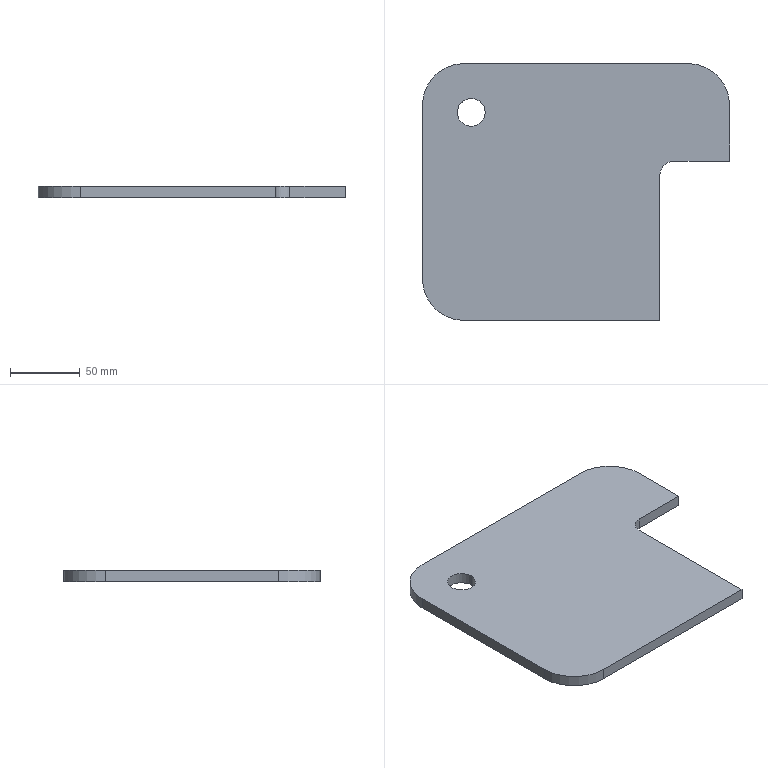Part | SolidWorks | features Extrusion 1 | 1 solid | 14 faces | box 220 x 184 x 8 mm | volume 271263 mm3 | plane 8 | cylinder 6 | commonest cylinder face diameters 20 x3 60 x3
STEP:
#1=CARTESIAN_POINT('',(25.,149.,8.));
#2=VERTEX_POINT('',#1);
#3=CARTESIAN_POINT('',(45.,149.,8.));
#4=VERTEX_POINT('',#3);
#5=CARTESIAN_POINT('',(35.,149.,8.));
#6=DIRECTION('',(0.,0.,1.));
#7=DIRECTION('',(1.,0.,0.));
#8=AXIS2_PLACEMENT_3D('',#5,#6,#7);
#9=CIRCLE('',#8,10.);
#10=EDGE_CURVE('',#2,#4,#9,.T.);
#11=ORIENTED_EDGE('',*,*,#10,.T.);
#12=CARTESIAN_POINT('',(45.,149.,0.));
#13=VERTEX_POINT('',#12);
#14=CARTESIAN_POINT('',(45.,149.,8.));
#15=DIRECTION('',(0.,0.,-1.));
#16=VECTOR('',#15,1000.);
#17=LINE('',#14,#16);
#18=EDGE_CURVE('',#4,#13,#17,.T.);
#19=ORIENTED_EDGE('',*,*,#18,.T.);
#20=CARTESIAN_POINT('',(25.,149.,0.));
#21=VERTEX_POINT('',#20);
#22=CARTESIAN_POINT('',(35.,149.,0.));
#23=DIRECTION('',(0.,0.,1.));
#24=DIRECTION('',(1.,0.,0.));
#25=AXIS2_PLACEMENT_3D('',#22,#23,#24);
#26=CIRCLE('',#25,10.);
#27=EDGE_CURVE('',#21,#13,#26,.T.);
#28=ORIENTED_EDGE('',*,*,#27,.F.);
#29=CARTESIAN_POINT('',(25.,149.,8.));
#30=DIRECTION('',(0.,0.,-1.));
#31=VECTOR('',#30,1000.);
#32=LINE('',#29,#31);
#33=EDGE_CURVE('',#2,#21,#32,.T.);
#34=ORIENTED_EDGE('',*,*,#33,.F.);
#35=EDGE_LOOP('',(#11,#19,#28,#34));
#36=FACE_OUTER_BOUND('',#35,.T.);
#37=CARTESIAN_POINT('',(35.,149.,8.));
#38=DIRECTION('',(0.,0.,-1.));
#39=DIRECTION('',(-1.,0.,0.));
#40=AXIS2_PLACEMENT_3D('',#37,#38,#39);
#41=CYLINDRICAL_SURFACE('',#40,10.);
#42=ADVANCED_FACE('',(#36),#41,.F.);
#43=CARTESIAN_POINT('',(220.,154.,8.));
#44=VERTEX_POINT('',#43);
#45=CARTESIAN_POINT('',(190.,184.,8.));
#46=VERTEX_POINT('',#45);
#47=CARTESIAN_POINT('',(190.,154.,8.));
#48=DIRECTION('',(0.,0.,1.));
#49=DIRECTION('',(-1.,0.,0.));
#50=AXIS2_PLACEMENT_3D('',#47,#48,#49);
#51=CIRCLE('',#50,30.);
#52=EDGE_CURVE('',#44,#46,#51,.T.);
#53=ORIENTED_EDGE('',*,*,#52,.T.);
#54=CARTESIAN_POINT('',(30.,184.,8.));
#55=VERTEX_POINT('',#54);
#56=CARTESIAN_POINT('',(30.,184.,8.));
#57=DIRECTION('',(-1.,0.,0.));
#58=VECTOR('',#57,1000.);
#59=LINE('',#56,#58);
#60=EDGE_CURVE('',#46,#55,#59,.T.);
#61=ORIENTED_EDGE('',*,*,#60,.T.);
#62=CARTESIAN_POINT('',(0.,154.,8.));
#63=VERTEX_POINT('',#62);
#64=CARTESIAN_POINT('',(30.,154.,8.));
#65=DIRECTION('',(0.,0.,1.));
#66=DIRECTION('',(-1.,0.,0.));
#67=AXIS2_PLACEMENT_3D('',#64,#65,#66);
#68=CIRCLE('',#67,30.);
#69=EDGE_CURVE('',#55,#63,#68,.T.);
#70=ORIENTED_EDGE('',*,*,#69,.T.);
#71=CARTESIAN_POINT('',(0.,30.,8.));
#72=VERTEX_POINT('',#71);
#73=CARTESIAN_POINT('',(0.,30.,8.));
#74=DIRECTION('',(0.,-1.,0.));
#75=VECTOR('',#74,1000.);
#76=LINE('',#73,#75);
#77=EDGE_CURVE('',#63,#72,#76,.T.);
#78=ORIENTED_EDGE('',*,*,#77,.T.);
#79=CARTESIAN_POINT('',(30.,0.,8.));
#80=VERTEX_POINT('',#79);
#81=CARTESIAN_POINT('',(30.,30.,8.));
#82=DIRECTION('',(0.,0.,1.));
#83=DIRECTION('',(1.,0.,0.));
#84=AXIS2_PLACEMENT_3D('',#81,#82,#83);
#85=CIRCLE('',#84,30.);
#86=EDGE_CURVE('',#72,#80,#85,.T.);
#87=ORIENTED_EDGE('',*,*,#86,.T.);
#88=CARTESIAN_POINT('',(170.,0.,8.));
#89=VERTEX_POINT('',#88);
#90=CARTESIAN_POINT('',(170.,0.,8.));
#91=DIRECTION('',(1.,0.,0.));
#92=VECTOR('',#91,1000.);
#93=LINE('',#90,#92);
#94=EDGE_CURVE('',#80,#89,#93,.T.);
#95=ORIENTED_EDGE('',*,*,#94,.T.);
#96=CARTESIAN_POINT('',(170.,104.,8.));
#97=VERTEX_POINT('',#96);
#98=CARTESIAN_POINT('',(170.,104.,8.));
#99=DIRECTION('',(0.,1.,0.));
#100=VECTOR('',#99,1000.);
#101=LINE('',#98,#100);
#102=EDGE_CURVE('',#89,#97,#101,.T.);
#103=ORIENTED_EDGE('',*,*,#102,.T.);
#104=CARTESIAN_POINT('',(180.,114.,8.));
#105=VERTEX_POINT('',#104);
#106=CARTESIAN_POINT('',(180.,104.,8.));
#107=DIRECTION('',(0.,0.,-1.));
#108=DIRECTION('',(1.,0.,0.));
#109=AXIS2_PLACEMENT_3D('',#106,#107,#108);
#110=CIRCLE('',#109,10.);
#111=EDGE_CURVE('',#97,#105,#110,.T.);
#112=ORIENTED_EDGE('',*,*,#111,.T.);
#113=CARTESIAN_POINT('',(220.,114.,8.));
#114=VERTEX_POINT('',#113);
#115=CARTESIAN_POINT('',(220.,114.,8.));
#116=DIRECTION('',(1.,0.,0.));
#117=VECTOR('',#116,1000.);
#118=LINE('',#115,#117);
#119=EDGE_CURVE('',#105,#114,#118,.T.);
#120=ORIENTED_EDGE('',*,*,#119,.T.);
#121=CARTESIAN_POINT('',(220.,154.,8.));
#122=DIRECTION('',(0.,1.,0.));
#123=VECTOR('',#122,1000.);
#124=LINE('',#121,#123);
#125=EDGE_CURVE('',#114,#44,#124,.T.);
#126=ORIENTED_EDGE('',*,*,#125,.T.);
#127=EDGE_LOOP('',(#53,#61,#70,#78,#87,#95,#103,#112,#120,#126));
#128=FACE_OUTER_BOUND('',#127,.T.);
#129=ORIENTED_EDGE('',*,*,#10,.F.);
#130=CARTESIAN_POINT('',(35.,149.,8.));
#131=DIRECTION('',(0.,0.,1.));
#132=DIRECTION('',(1.,0.,0.));
#133=AXIS2_PLACEMENT_3D('',#130,#131,#132);
#134=CIRCLE('',#133,10.);
#135=EDGE_CURVE('',#4,#2,#134,.T.);
#136=ORIENTED_EDGE('',*,*,#135,.F.);
#137=EDGE_LOOP('',(#129,#136));
#138=FACE_BOUND('',#137,.T.);
#139=CARTESIAN_POINT('',(190.,154.,8.));
#140=DIRECTION('',(0.,0.,-1.));
#141=DIRECTION('',(-1.,0.,0.));
#142=AXIS2_PLACEMENT_3D('',#139,#140,#141);
#143=PLANE('',#142);
#144=ADVANCED_FACE('',(#128,#138),#143,.F.);
#145=CARTESIAN_POINT('',(220.,154.,0.));
#146=VERTEX_POINT('',#145);
#147=CARTESIAN_POINT('',(190.,184.,0.));
#148=VERTEX_POINT('',#147);
#149=CARTESIAN_POINT('',(190.,154.,0.));
#150=DIRECTION('',(0.,0.,1.));
#151=DIRECTION('',(-1.,0.,0.));
#152=AXIS2_PLACEMENT_3D('',#149,#150,#151);
#153=CIRCLE('',#152,30.);
#154=EDGE_CURVE('',#146,#148,#153,.T.);
#155=ORIENTED_EDGE('',*,*,#154,.F.);
#156=CARTESIAN_POINT('',(220.,114.,0.));
#157=VERTEX_POINT('',#156);
#158=CARTESIAN_POINT('',(220.,154.,0.));
#159=DIRECTION('',(0.,1.,0.));
#160=VECTOR('',#159,1000.);
#161=LINE('',#158,#160);
#162=EDGE_CURVE('',#157,#146,#161,.T.);
#163=ORIENTED_EDGE('',*,*,#162,.F.);
#164=CARTESIAN_POINT('',(180.,114.,0.));
#165=VERTEX_POINT('',#164);
#166=CARTESIAN_POINT('',(220.,114.,0.));
#167=DIRECTION('',(1.,0.,0.));
#168=VECTOR('',#167,1000.);
#169=LINE('',#166,#168);
#170=EDGE_CURVE('',#165,#157,#169,.T.);
#171=ORIENTED_EDGE('',*,*,#170,.F.);
#172=CARTESIAN_POINT('',(170.,104.,0.));
#173=VERTEX_POINT('',#172);
#174=CARTESIAN_POINT('',(180.,104.,0.));
#175=DIRECTION('',(0.,0.,-1.));
#176=DIRECTION('',(1.,0.,0.));
#177=AXIS2_PLACEMENT_3D('',#174,#175,#176);
#178=CIRCLE('',#177,10.);
#179=EDGE_CURVE('',#173,#165,#178,.T.);
#180=ORIENTED_EDGE('',*,*,#179,.F.);
#181=CARTESIAN_POINT('',(170.,0.,0.));
#182=VERTEX_POINT('',#181);
#183=CARTESIAN_POINT('',(170.,104.,0.));
#184=DIRECTION('',(0.,1.,0.));
#185=VECTOR('',#184,1000.);
#186=LINE('',#183,#185);
#187=EDGE_CURVE('',#182,#173,#186,.T.);
#188=ORIENTED_EDGE('',*,*,#187,.F.);
#189=CARTESIAN_POINT('',(30.,0.,0.));
#190=VERTEX_POINT('',#189);
#191=CARTESIAN_POINT('',(170.,0.,0.));
#192=DIRECTION('',(1.,0.,0.));
#193=VECTOR('',#192,1000.);
#194=LINE('',#191,#193);
#195=EDGE_CURVE('',#190,#182,#194,.T.);
#196=ORIENTED_EDGE('',*,*,#195,.F.);
#197=CARTESIAN_POINT('',(0.,30.,0.));
#198=VERTEX_POINT('',#197);
#199=CARTESIAN_POINT('',(30.,30.,0.));
#200=DIRECTION('',(0.,0.,1.));
#201=DIRECTION('',(1.,0.,0.));
#202=AXIS2_PLACEMENT_3D('',#199,#200,#201);
#203=CIRCLE('',#202,30.);
#204=EDGE_CURVE('',#198,#190,#203,.T.);
#205=ORIENTED_EDGE('',*,*,#204,.F.);
#206=CARTESIAN_POINT('',(0.,154.,0.));
#207=VERTEX_POINT('',#206);
#208=CARTESIAN_POINT('',(0.,30.,0.));
#209=DIRECTION('',(0.,-1.,0.));
#210=VECTOR('',#209,1000.);
#211=LINE('',#208,#210);
#212=EDGE_CURVE('',#207,#198,#211,.T.);
#213=ORIENTED_EDGE('',*,*,#212,.F.);
#214=CARTESIAN_POINT('',(30.,184.,0.));
#215=VERTEX_POINT('',#214);
#216=CARTESIAN_POINT('',(30.,154.,0.));
#217=DIRECTION('',(0.,0.,1.));
#218=DIRECTION('',(-1.,0.,0.));
#219=AXIS2_PLACEMENT_3D('',#216,#217,#218);
#220=CIRCLE('',#219,30.);
#221=EDGE_CURVE('',#215,#207,#220,.T.);
#222=ORIENTED_EDGE('',*,*,#221,.F.);
#223=CARTESIAN_POINT('',(30.,184.,0.));
#224=DIRECTION('',(-1.,0.,0.));
#225=VECTOR('',#224,1000.);
#226=LINE('',#223,#225);
#227=EDGE_CURVE('',#148,#215,#226,.T.);
#228=ORIENTED_EDGE('',*,*,#227,.F.);
#229=EDGE_LOOP('',(#155,#163,#171,#180,#188,#196,#205,#213,#222,#228));
#230=FACE_OUTER_BOUND('',#229,.T.);
#231=ORIENTED_EDGE('',*,*,#27,.T.);
#232=CARTESIAN_POINT('',(35.,149.,0.));
#233=DIRECTION('',(0.,0.,1.));
#234=DIRECTION('',(1.,0.,0.));
#235=AXIS2_PLACEMENT_3D('',#232,#233,#234);
#236=CIRCLE('',#235,10.);
#237=EDGE_CURVE('',#13,#21,#236,.T.);
#238=ORIENTED_EDGE('',*,*,#237,.T.);
#239=EDGE_LOOP('',(#231,#238));
#240=FACE_BOUND('',#239,.T.);
#241=CARTESIAN_POINT('',(190.,154.,0.));
#242=DIRECTION('',(0.,0.,-1.));
#243=DIRECTION('',(-1.,0.,0.));
#244=AXIS2_PLACEMENT_3D('',#241,#242,#243);
#245=PLANE('',#244);
#246=ADVANCED_FACE('',(#230,#240),#245,.T.);
#247=ORIENTED_EDGE('',*,*,#154,.T.);
#248=CARTESIAN_POINT('',(190.,184.,8.));
#249=DIRECTION('',(0.,0.,-1.));
#250=VECTOR('',#249,1000.);
#251=LINE('',#248,#250);
#252=EDGE_CURVE('',#46,#148,#251,.T.);
#253=ORIENTED_EDGE('',*,*,#252,.F.);
#254=ORIENTED_EDGE('',*,*,#52,.F.);
#255=CARTESIAN_POINT('',(220.,154.,8.));
#256=DIRECTION('',(0.,0.,-1.));
#257=VECTOR('',#256,1000.);
#258=LINE('',#255,#257);
#259=EDGE_CURVE('',#44,#146,#258,.T.);
#260=ORIENTED_EDGE('',*,*,#259,.T.);
#261=EDGE_LOOP('',(#247,#253,#254,#260));
#262=FACE_OUTER_BOUND('',#261,.T.);
#263=CARTESIAN_POINT('',(190.,154.,8.));
#264=DIRECTION('',(0.,0.,-1.));
#265=DIRECTION('',(-1.,0.,0.));
#266=AXIS2_PLACEMENT_3D('',#263,#264,#265);
#267=CYLINDRICAL_SURFACE('',#266,30.);
#268=ADVANCED_FACE('',(#262),#267,.T.);
#269=ORIENTED_EDGE('',*,*,#227,.T.);
#270=CARTESIAN_POINT('',(30.,184.,8.));
#271=DIRECTION('',(0.,0.,-1.));
#272=VECTOR('',#271,1000.);
#273=LINE('',#270,#272);
#274=EDGE_CURVE('',#55,#215,#273,.T.);
#275=ORIENTED_EDGE('',*,*,#274,.F.);
#276=ORIENTED_EDGE('',*,*,#60,.F.);
#277=ORIENTED_EDGE('',*,*,#252,.T.);
#278=EDGE_LOOP('',(#269,#275,#276,#277));
#279=FACE_OUTER_BOUND('',#278,.T.);
#280=CARTESIAN_POINT('',(30.,184.,8.));
#281=DIRECTION('',(0.,-1.,0.));
#282=DIRECTION('',(0.,0.,-1.));
#283=AXIS2_PLACEMENT_3D('',#280,#281,#282);
#284=PLANE('',#283);
#285=ADVANCED_FACE('',(#279),#284,.F.);
#286=ORIENTED_EDGE('',*,*,#221,.T.);
#287=CARTESIAN_POINT('',(0.,154.,8.));
#288=DIRECTION('',(0.,0.,-1.));
#289=VECTOR('',#288,1000.);
#290=LINE('',#287,#289);
#291=EDGE_CURVE('',#63,#207,#290,.T.);
#292=ORIENTED_EDGE('',*,*,#291,.F.);
#293=ORIENTED_EDGE('',*,*,#69,.F.);
#294=ORIENTED_EDGE('',*,*,#274,.T.);
#295=EDGE_LOOP('',(#286,#292,#293,#294));
#296=FACE_OUTER_BOUND('',#295,.T.);
#297=CARTESIAN_POINT('',(30.,154.,8.));
#298=DIRECTION('',(0.,0.,-1.));
#299=DIRECTION('',(-1.,0.,0.));
#300=AXIS2_PLACEMENT_3D('',#297,#298,#299);
#301=CYLINDRICAL_SURFACE('',#300,30.);
#302=ADVANCED_FACE('',(#296),#301,.T.);
#303=ORIENTED_EDGE('',*,*,#212,.T.);
#304=CARTESIAN_POINT('',(0.,30.,8.));
#305=DIRECTION('',(0.,0.,-1.));
#306=VECTOR('',#305,1000.);
#307=LINE('',#304,#306);
#308=EDGE_CURVE('',#72,#198,#307,.T.);
#309=ORIENTED_EDGE('',*,*,#308,.F.);
#310=ORIENTED_EDGE('',*,*,#77,.F.);
#311=ORIENTED_EDGE('',*,*,#291,.T.);
#312=EDGE_LOOP('',(#303,#309,#310,#311));
#313=FACE_OUTER_BOUND('',#312,.T.);
#314=CARTESIAN_POINT('',(0.,30.,8.));
#315=DIRECTION('',(1.,0.,0.));
#316=DIRECTION('',(0.,0.,-1.));
#317=AXIS2_PLACEMENT_3D('',#314,#315,#316);
#318=PLANE('',#317);
#319=ADVANCED_FACE('',(#313),#318,.F.);
#320=ORIENTED_EDGE('',*,*,#204,.T.);
#321=CARTESIAN_POINT('',(30.,0.,8.));
#322=DIRECTION('',(0.,0.,-1.));
#323=VECTOR('',#322,1000.);
#324=LINE('',#321,#323);
#325=EDGE_CURVE('',#80,#190,#324,.T.);
#326=ORIENTED_EDGE('',*,*,#325,.F.);
#327=ORIENTED_EDGE('',*,*,#86,.F.);
#328=ORIENTED_EDGE('',*,*,#308,.T.);
#329=EDGE_LOOP('',(#320,#326,#327,#328));
#330=FACE_OUTER_BOUND('',#329,.T.);
#331=CARTESIAN_POINT('',(30.,30.,8.));
#332=DIRECTION('',(0.,0.,-1.));
#333=DIRECTION('',(-1.,0.,0.));
#334=AXIS2_PLACEMENT_3D('',#331,#332,#333);
#335=CYLINDRICAL_SURFACE('',#334,30.);
#336=ADVANCED_FACE('',(#330),#335,.T.);
#337=ORIENTED_EDGE('',*,*,#195,.T.);
#338=CARTESIAN_POINT('',(170.,0.,8.));
#339=DIRECTION('',(0.,0.,-1.));
#340=VECTOR('',#339,1000.);
#341=LINE('',#338,#340);
#342=EDGE_CURVE('',#89,#182,#341,.T.);
#343=ORIENTED_EDGE('',*,*,#342,.F.);
#344=ORIENTED_EDGE('',*,*,#94,.F.);
#345=ORIENTED_EDGE('',*,*,#325,.T.);
#346=EDGE_LOOP('',(#337,#343,#344,#345));
#347=FACE_OUTER_BOUND('',#346,.T.);
#348=CARTESIAN_POINT('',(170.,0.,8.));
#349=DIRECTION('',(0.,1.,0.));
#350=DIRECTION('',(-1.,0.,0.));
#351=AXIS2_PLACEMENT_3D('',#348,#349,#350);
#352=PLANE('',#351);
#353=ADVANCED_FACE('',(#347),#352,.F.);
#354=ORIENTED_EDGE('',*,*,#187,.T.);
#355=CARTESIAN_POINT('',(170.,104.,8.));
#356=DIRECTION('',(0.,0.,-1.));
#357=VECTOR('',#356,1000.);
#358=LINE('',#355,#357);
#359=EDGE_CURVE('',#97,#173,#358,.T.);
#360=ORIENTED_EDGE('',*,*,#359,.F.);
#361=ORIENTED_EDGE('',*,*,#102,.F.);
#362=ORIENTED_EDGE('',*,*,#342,.T.);
#363=EDGE_LOOP('',(#354,#360,#361,#362));
#364=FACE_OUTER_BOUND('',#363,.T.);
#365=CARTESIAN_POINT('',(170.,104.,8.));
#366=DIRECTION('',(-1.,0.,0.));
#367=DIRECTION('',(0.,0.,1.));
#368=AXIS2_PLACEMENT_3D('',#365,#366,#367);
#369=PLANE('',#368);
#370=ADVANCED_FACE('',(#364),#369,.F.);
#371=ORIENTED_EDGE('',*,*,#179,.T.);
#372=CARTESIAN_POINT('',(180.,114.,8.));
#373=DIRECTION('',(0.,0.,-1.));
#374=VECTOR('',#373,1000.);
#375=LINE('',#372,#374);
#376=EDGE_CURVE('',#105,#165,#375,.T.);
#377=ORIENTED_EDGE('',*,*,#376,.F.);
#378=ORIENTED_EDGE('',*,*,#111,.F.);
#379=ORIENTED_EDGE('',*,*,#359,.T.);
#380=EDGE_LOOP('',(#371,#377,#378,#379));
#381=FACE_OUTER_BOUND('',#380,.T.);
#382=CARTESIAN_POINT('',(180.,104.,8.));
#383=DIRECTION('',(0.,0.,-1.));
#384=DIRECTION('',(-1.,0.,0.));
#385=AXIS2_PLACEMENT_3D('',#382,#383,#384);
#386=CYLINDRICAL_SURFACE('',#385,10.);
#387=ADVANCED_FACE('',(#381),#386,.F.);
#388=ORIENTED_EDGE('',*,*,#170,.T.);
#389=CARTESIAN_POINT('',(220.,114.,8.));
#390=DIRECTION('',(0.,0.,-1.));
#391=VECTOR('',#390,1000.);
#392=LINE('',#389,#391);
#393=EDGE_CURVE('',#114,#157,#392,.T.);
#394=ORIENTED_EDGE('',*,*,#393,.F.);
#395=ORIENTED_EDGE('',*,*,#119,.F.);
#396=ORIENTED_EDGE('',*,*,#376,.T.);
#397=EDGE_LOOP('',(#388,#394,#395,#396));
#398=FACE_OUTER_BOUND('',#397,.T.);
#399=CARTESIAN_POINT('',(220.,114.,8.));
#400=DIRECTION('',(0.,1.,0.));
#401=DIRECTION('',(-1.,0.,0.));
#402=AXIS2_PLACEMENT_3D('',#399,#400,#401);
#403=PLANE('',#402);
#404=ADVANCED_FACE('',(#398),#403,.F.);
#405=ORIENTED_EDGE('',*,*,#162,.T.);
#406=ORIENTED_EDGE('',*,*,#259,.F.);
#407=ORIENTED_EDGE('',*,*,#125,.F.);
#408=ORIENTED_EDGE('',*,*,#393,.T.);
#409=EDGE_LOOP('',(#405,#406,#407,#408));
#410=FACE_OUTER_BOUND('',#409,.T.);
#411=CARTESIAN_POINT('',(220.,154.,8.));
#412=DIRECTION('',(-1.,0.,0.));
#413=DIRECTION('',(0.,0.,1.));
#414=AXIS2_PLACEMENT_3D('',#411,#412,#413);
#415=PLANE('',#414);
#416=ADVANCED_FACE('',(#410),#415,.F.);
#417=ORIENTED_EDGE('',*,*,#18,.F.);
#418=ORIENTED_EDGE('',*,*,#135,.T.);
#419=ORIENTED_EDGE('',*,*,#33,.T.);
#420=ORIENTED_EDGE('',*,*,#237,.F.);
#421=EDGE_LOOP('',(#417,#418,#419,#420));
#422=FACE_OUTER_BOUND('',#421,.T.);
#423=CARTESIAN_POINT('',(35.,149.,8.));
#424=DIRECTION('',(0.,0.,-1.));
#425=DIRECTION('',(-1.,0.,0.));
#426=AXIS2_PLACEMENT_3D('',#423,#424,#425);
#427=CYLINDRICAL_SURFACE('',#426,10.);
#428=ADVANCED_FACE('',(#422),#427,.F.);
#429=CLOSED_SHELL('',(#42,#144,#246,#268,#285,#302,#319,#336,#353,#370,#387,#404,#416,#428));
#430=MANIFOLD_SOLID_BREP('',#429);
#431=CARTESIAN_POINT('',(0.,0.,0.));
#432=DIRECTION('',(0.,0.,1.));
#433=DIRECTION('',(1.,0.,0.));
#434=AXIS2_PLACEMENT_3D('',#431,#432,#433);
#435=(LENGTH_UNIT()NAMED_UNIT(*)SI_UNIT(.MILLI.,.METRE.));
#436=UNCERTAINTY_MEASURE_WITH_UNIT(LENGTH_MEASURE(0.00001),#435,'','');
#437=(NAMED_UNIT(*)PLANE_ANGLE_UNIT()SI_UNIT($,.RADIAN.));
#438=(NAMED_UNIT(*)SI_UNIT($,.STERADIAN.)SOLID_ANGLE_UNIT());
#439=(GEOMETRIC_REPRESENTATION_CONTEXT(3)GLOBAL_UNCERTAINTY_ASSIGNED_CONTEXT((#436))GLOBAL_UNIT_ASSIGNED_CONTEXT((#435,#437,#438))REPRESENTATION_CONTEXT('',''));
#440=ADVANCED_BREP_SHAPE_REPRESENTATION('',(#430,#434),#439);